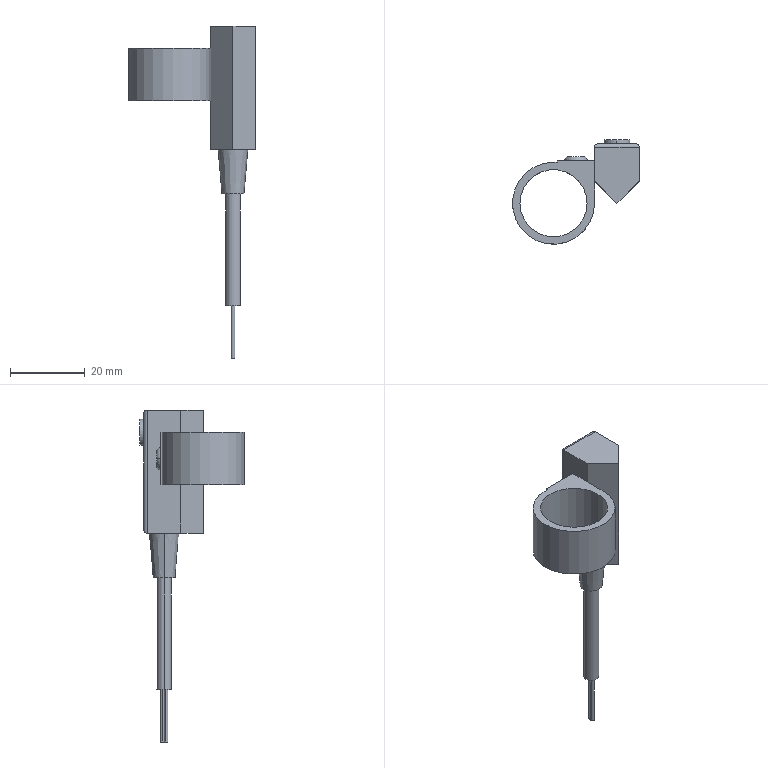Part | STEP file | CDS1FN180-250-A54Z_A5_A6_F5_J5_ForLargeBore | 1 solid | 44 faces | box 34 x 28 x 89 mm | volume 8233 mm3 | plane 23 | cylinder 17 | torus 2 | cone 2 | commonest cylinder face diameters 1 x4 2 x4 3 x2 4 x2 7 x2 18 x2